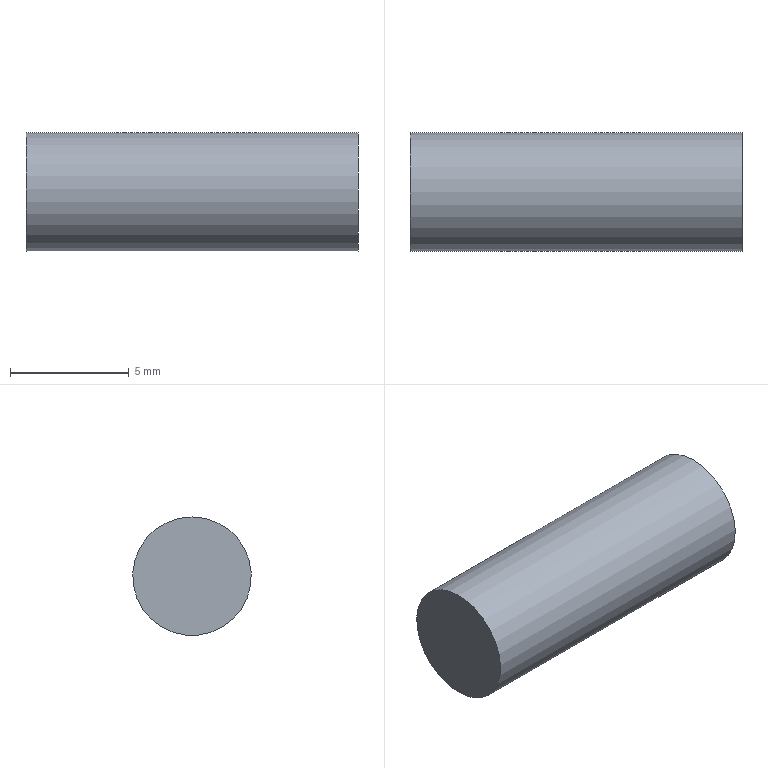Part | NX | features solid 2 | 1 solid | 3 faces | box 14 x 5 x 5 mm | volume 274.889 mm3 | plane 2 | cylinder 1 | commonest cylinder face diameters 5 x1
STEP:
#1=CARTESIAN_POINT('',(-22.,0.,138.));
#2=VERTEX_POINT('',#1);
#3=CARTESIAN_POINT('',(-22.,0.,135.5));
#4=DIRECTION('',(1.,0.,0.));
#5=DIRECTION('',(0.,0.,1.));
#6=AXIS2_PLACEMENT_3D('',#3,#4,#5);
#7=CIRCLE('',#6,2.5);
#8=EDGE_CURVE('',#2,#2,#7,.T.);
#9=ORIENTED_EDGE('',*,*,#8,.F.);
#10=EDGE_LOOP('',(#9));
#11=FACE_BOUND('',#10,.T.);
#12=CARTESIAN_POINT('',(-22.,0.,135.5));
#13=DIRECTION('',(-1.,0.,0.));
#14=DIRECTION('',(0.,-1.,0.));
#15=AXIS2_PLACEMENT_3D('',#12,#13,#14);
#16=PLANE('',#15);
#17=ADVANCED_FACE('',(#11),#16,.T.);
#18=CARTESIAN_POINT('',(-8.,0.,138.));
#19=VERTEX_POINT('',#18);
#20=CARTESIAN_POINT('',(-8.,0.,135.5));
#21=DIRECTION('',(-1.,0.,0.));
#22=DIRECTION('',(0.,0.,1.));
#23=AXIS2_PLACEMENT_3D('',#20,#21,#22);
#24=CIRCLE('',#23,2.5);
#25=EDGE_CURVE('',#19,#19,#24,.T.);
#26=ORIENTED_EDGE('',*,*,#25,.F.);
#27=EDGE_LOOP('',(#26));
#28=FACE_BOUND('',#27,.T.);
#29=CARTESIAN_POINT('',(-8.,0.,135.5));
#30=DIRECTION('',(1.,0.,0.));
#31=DIRECTION('',(0.,1.,0.));
#32=AXIS2_PLACEMENT_3D('',#29,#30,#31);
#33=PLANE('',#32);
#34=ADVANCED_FACE('',(#28),#33,.T.);
#35=ORIENTED_EDGE('',*,*,#8,.T.);
#36=EDGE_LOOP('',(#35));
#37=FACE_BOUND('',#36,.T.);
#38=ORIENTED_EDGE('',*,*,#25,.T.);
#39=EDGE_LOOP('',(#38));
#40=FACE_BOUND('',#39,.T.);
#41=CARTESIAN_POINT('',(-8.,0.,135.5));
#42=DIRECTION('',(-1.,0.,0.));
#43=DIRECTION('',(0.,0.,1.));
#44=AXIS2_PLACEMENT_3D('',#41,#42,#43);
#45=CYLINDRICAL_SURFACE('',#44,2.5);
#46=ADVANCED_FACE('',(#37,#40),#45,.T.);
#47=CLOSED_SHELL('',(#17,#34,#46));
#48=MANIFOLD_SOLID_BREP('',#47);
#49=(LENGTH_UNIT()NAMED_UNIT(*)SI_UNIT(.MILLI.,.METRE.));
#50=UNCERTAINTY_MEASURE_WITH_UNIT(LENGTH_MEASURE(0.00001),#49,'','');
#51=(NAMED_UNIT(*)PLANE_ANGLE_UNIT()SI_UNIT($,.RADIAN.));
#52=(NAMED_UNIT(*)SI_UNIT($,.STERADIAN.)SOLID_ANGLE_UNIT());
#53=(GEOMETRIC_REPRESENTATION_CONTEXT(3)GLOBAL_UNCERTAINTY_ASSIGNED_CONTEXT((#50))GLOBAL_UNIT_ASSIGNED_CONTEXT((#49,#51,#52))REPRESENTATION_CONTEXT('',''));
#54=ADVANCED_BREP_SHAPE_REPRESENTATION('',(#48),#53);